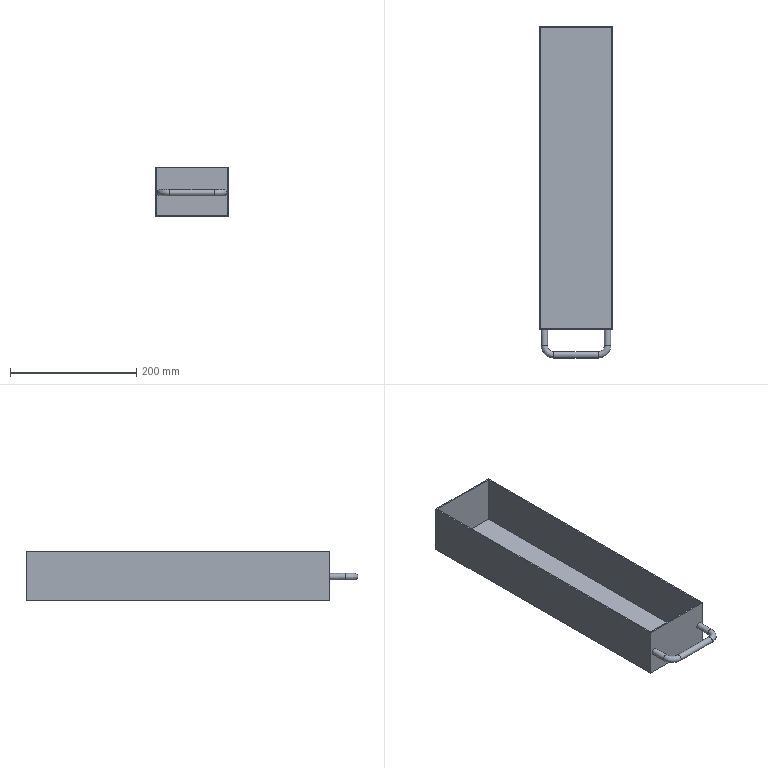Part | NX | features solid 2 | 1 solid | 16 faces | box 117 x 525 x 78 mm | volume 305718 mm3 | plane 11 | cylinder 3 | torus 2 | commonest cylinder face diameters 10 x3
STEP:
#1=CARTESIAN_POINT('',(-337.5,-405.,-285.));
#2=VERTEX_POINT('',#1);
#3=CARTESIAN_POINT('',(-337.5,-405.,-280.));
#4=DIRECTION('',(0.,-1.,0.));
#5=DIRECTION('',(0.,0.,-1.));
#6=AXIS2_PLACEMENT_3D('',#3,#4,#5);
#7=CIRCLE('',#6,5.);
#8=EDGE_CURVE('',#2,#2,#7,.T.);
#9=ORIENTED_EDGE('',*,*,#8,.F.);
#10=EDGE_LOOP('',(#9));
#11=FACE_BOUND('',#10,.T.);
#12=CARTESIAN_POINT('',(-346.,-405.,-240.));
#13=VERTEX_POINT('',#12);
#14=CARTESIAN_POINT('',(-229.,-405.,-240.));
#15=VERTEX_POINT('',#14);
#16=CARTESIAN_POINT('',(-350.,-405.,-240.));
#17=DIRECTION('',(1.,0.,0.));
#18=VECTOR('',#17,1000.);
#19=LINE('',#16,#18);
#20=EDGE_CURVE('',#13,#15,#19,.T.);
#21=ORIENTED_EDGE('',*,*,#20,.F.);
#22=CARTESIAN_POINT('',(-346.,-405.,-318.));
#23=VERTEX_POINT('',#22);
#24=CARTESIAN_POINT('',(-346.,-405.,0.));
#25=DIRECTION('',(0.,0.,1.));
#26=VECTOR('',#25,1000.);
#27=LINE('',#24,#26);
#28=EDGE_CURVE('',#23,#13,#27,.T.);
#29=ORIENTED_EDGE('',*,*,#28,.F.);
#30=CARTESIAN_POINT('',(-229.,-405.,-318.));
#31=VERTEX_POINT('',#30);
#32=CARTESIAN_POINT('',(-350.,-405.,-318.));
#33=DIRECTION('',(-1.,0.,0.));
#34=VECTOR('',#33,1000.);
#35=LINE('',#32,#34);
#36=EDGE_CURVE('',#23,#31,#35,.F.);
#37=ORIENTED_EDGE('',*,*,#36,.T.);
#38=CARTESIAN_POINT('',(-229.,-405.,-85.));
#39=DIRECTION('',(0.,0.,1.));
#40=VECTOR('',#39,1000.);
#41=LINE('',#38,#40);
#42=EDGE_CURVE('',#31,#15,#41,.T.);
#43=ORIENTED_EDGE('',*,*,#42,.T.);
#44=EDGE_LOOP('',(#21,#29,#37,#43));
#45=FACE_BOUND('',#44,.T.);
#46=CARTESIAN_POINT('',(-242.5,-405.,-280.));
#47=VERTEX_POINT('',#46);
#48=CARTESIAN_POINT('',(-237.5,-405.,-280.));
#49=DIRECTION('',(0.,-1.,0.));
#50=DIRECTION('',(-1.,0.,0.));
#51=AXIS2_PLACEMENT_3D('',#48,#49,#50);
#52=CIRCLE('',#51,5.);
#53=EDGE_CURVE('',#47,#47,#52,.T.);
#54=ORIENTED_EDGE('',*,*,#53,.F.);
#55=EDGE_LOOP('',(#54));
#56=FACE_BOUND('',#55,.T.);
#57=CARTESIAN_POINT('',(-910.,-405.,-85.));
#58=DIRECTION('',(0.,-1.,0.));
#59=DIRECTION('',(0.,0.,-1.));
#60=AXIS2_PLACEMENT_3D('',#57,#58,#59);
#61=PLANE('',#60);
#62=ADVANCED_FACE('',(#11,#45,#56),#61,.T.);
#63=CARTESIAN_POINT('',(-229.,75.,-240.));
#64=VERTEX_POINT('',#63);
#65=CARTESIAN_POINT('',(-346.,75.,-240.));
#66=VERTEX_POINT('',#65);
#67=CARTESIAN_POINT('',(-350.,75.,-240.));
#68=DIRECTION('',(1.,0.,0.));
#69=VECTOR('',#68,1000.);
#70=LINE('',#67,#69);
#71=EDGE_CURVE('',#64,#66,#70,.F.);
#72=ORIENTED_EDGE('',*,*,#71,.F.);
#73=CARTESIAN_POINT('',(-229.,75.,-318.));
#74=VERTEX_POINT('',#73);
#75=CARTESIAN_POINT('',(-229.,75.,0.));
#76=DIRECTION('',(0.,0.,-1.));
#77=VECTOR('',#76,1000.);
#78=LINE('',#75,#77);
#79=EDGE_CURVE('',#74,#64,#78,.F.);
#80=ORIENTED_EDGE('',*,*,#79,.F.);
#81=CARTESIAN_POINT('',(-346.,75.,-318.));
#82=VERTEX_POINT('',#81);
#83=CARTESIAN_POINT('',(-350.,75.,-318.));
#84=DIRECTION('',(-1.,0.,0.));
#85=VECTOR('',#84,1000.);
#86=LINE('',#83,#85);
#87=EDGE_CURVE('',#74,#82,#86,.T.);
#88=ORIENTED_EDGE('',*,*,#87,.T.);
#89=CARTESIAN_POINT('',(-346.,75.,-320.));
#90=DIRECTION('',(0.,0.,-1.));
#91=VECTOR('',#90,1000.);
#92=LINE('',#89,#91);
#93=EDGE_CURVE('',#82,#66,#92,.F.);
#94=ORIENTED_EDGE('',*,*,#93,.T.);
#95=EDGE_LOOP('',(#72,#80,#88,#94));
#96=FACE_BOUND('',#95,.T.);
#97=CARTESIAN_POINT('',(-225.,75.,-320.));
#98=DIRECTION('',(0.,-1.,0.));
#99=DIRECTION('',(-1.,0.,0.));
#100=AXIS2_PLACEMENT_3D('',#97,#98,#99);
#101=PLANE('',#100);
#102=ADVANCED_FACE('',(#96),#101,.F.);
#103=CARTESIAN_POINT('',(-346.,105.,-240.));
#104=DIRECTION('',(0.,-1.,0.));
#105=VECTOR('',#104,1000.);
#106=LINE('',#103,#105);
#107=EDGE_CURVE('',#66,#13,#106,.T.);
#108=ORIENTED_EDGE('',*,*,#107,.F.);
#109=ORIENTED_EDGE('',*,*,#93,.F.);
#110=CARTESIAN_POINT('',(-346.,-70.,-318.));
#111=DIRECTION('',(0.,1.,0.));
#112=VECTOR('',#111,1000.);
#113=LINE('',#110,#112);
#114=EDGE_CURVE('',#82,#23,#113,.F.);
#115=ORIENTED_EDGE('',*,*,#114,.T.);
#116=ORIENTED_EDGE('',*,*,#28,.T.);
#117=EDGE_LOOP('',(#108,#109,#115,#116));
#118=FACE_BOUND('',#117,.T.);
#119=CARTESIAN_POINT('',(-346.,105.,0.));
#120=DIRECTION('',(-1.,0.,0.));
#121=DIRECTION('',(0.,0.,1.));
#122=AXIS2_PLACEMENT_3D('',#119,#120,#121);
#123=PLANE('',#122);
#124=ADVANCED_FACE('',(#118),#123,.T.);
#125=CARTESIAN_POINT('',(-229.,105.,-240.));
#126=DIRECTION('',(0.,1.,0.));
#127=VECTOR('',#126,1000.);
#128=LINE('',#125,#127);
#129=EDGE_CURVE('',#15,#64,#128,.T.);
#130=ORIENTED_EDGE('',*,*,#129,.F.);
#131=ORIENTED_EDGE('',*,*,#42,.F.);
#132=CARTESIAN_POINT('',(-229.,-70.,-318.));
#133=DIRECTION('',(0.,-1.,0.));
#134=VECTOR('',#133,1000.);
#135=LINE('',#132,#134);
#136=EDGE_CURVE('',#31,#74,#135,.F.);
#137=ORIENTED_EDGE('',*,*,#136,.T.);
#138=ORIENTED_EDGE('',*,*,#79,.T.);
#139=EDGE_LOOP('',(#130,#131,#137,#138));
#140=FACE_BOUND('',#139,.T.);
#141=CARTESIAN_POINT('',(-229.,-400.,0.));
#142=DIRECTION('',(1.,0.,0.));
#143=DIRECTION('',(0.,0.,-1.));
#144=AXIS2_PLACEMENT_3D('',#141,#142,#143);
#145=PLANE('',#144);
#146=ADVANCED_FACE('',(#140),#145,.T.);
#147=ORIENTED_EDGE('',*,*,#87,.F.);
#148=ORIENTED_EDGE('',*,*,#136,.F.);
#149=ORIENTED_EDGE('',*,*,#36,.F.);
#150=ORIENTED_EDGE('',*,*,#114,.F.);
#151=EDGE_LOOP('',(#147,#148,#149,#150));
#152=FACE_BOUND('',#151,.T.);
#153=CARTESIAN_POINT('',(-350.,-70.,-318.));
#154=DIRECTION('',(0.,0.,-1.));
#155=DIRECTION('',(-1.,0.,0.));
#156=AXIS2_PLACEMENT_3D('',#153,#154,#155);
#157=PLANE('',#156);
#158=ADVANCED_FACE('',(#152),#157,.T.);
#159=CARTESIAN_POINT('',(-231.,73.,-240.));
#160=VERTEX_POINT('',#159);
#161=CARTESIAN_POINT('',(-344.,73.,-240.));
#162=VERTEX_POINT('',#161);
#163=CARTESIAN_POINT('',(-350.,73.,-240.));
#164=DIRECTION('',(1.,0.,0.));
#165=VECTOR('',#164,1000.);
#166=LINE('',#163,#165);
#167=EDGE_CURVE('',#160,#162,#166,.F.);
#168=ORIENTED_EDGE('',*,*,#167,.F.);
#169=CARTESIAN_POINT('',(-231.,-403.,-240.));
#170=VERTEX_POINT('',#169);
#171=CARTESIAN_POINT('',(-231.,105.,-240.));
#172=DIRECTION('',(0.,1.,0.));
#173=VECTOR('',#172,1000.);
#174=LINE('',#171,#173);
#175=EDGE_CURVE('',#170,#160,#174,.T.);
#176=ORIENTED_EDGE('',*,*,#175,.F.);
#177=CARTESIAN_POINT('',(-344.,-403.,-240.));
#178=VERTEX_POINT('',#177);
#179=CARTESIAN_POINT('',(-350.,-403.,-240.));
#180=DIRECTION('',(1.,0.,0.));
#181=VECTOR('',#180,1000.);
#182=LINE('',#179,#181);
#183=EDGE_CURVE('',#178,#170,#182,.T.);
#184=ORIENTED_EDGE('',*,*,#183,.F.);
#185=CARTESIAN_POINT('',(-344.,105.,-240.));
#186=DIRECTION('',(0.,-1.,0.));
#187=VECTOR('',#186,1000.);
#188=LINE('',#185,#187);
#189=EDGE_CURVE('',#162,#178,#188,.T.);
#190=ORIENTED_EDGE('',*,*,#189,.F.);
#191=EDGE_LOOP('',(#168,#176,#184,#190));
#192=FACE_BOUND('',#191,.T.);
#193=ORIENTED_EDGE('',*,*,#71,.T.);
#194=ORIENTED_EDGE('',*,*,#107,.T.);
#195=ORIENTED_EDGE('',*,*,#20,.T.);
#196=ORIENTED_EDGE('',*,*,#129,.T.);
#197=EDGE_LOOP('',(#193,#194,#195,#196));
#198=FACE_BOUND('',#197,.T.);
#199=CARTESIAN_POINT('',(-350.,105.,-240.));
#200=DIRECTION('',(0.,0.,1.));
#201=DIRECTION('',(1.,0.,0.));
#202=AXIS2_PLACEMENT_3D('',#199,#200,#201);
#203=PLANE('',#202);
#204=ADVANCED_FACE('',(#192,#198),#203,.T.);
#205=ORIENTED_EDGE('',*,*,#167,.T.);
#206=CARTESIAN_POINT('',(-344.,73.,-316.));
#207=VERTEX_POINT('',#206);
#208=CARTESIAN_POINT('',(-344.,73.,-320.));
#209=DIRECTION('',(0.,0.,-1.));
#210=VECTOR('',#209,1000.);
#211=LINE('',#208,#210);
#212=EDGE_CURVE('',#207,#162,#211,.F.);
#213=ORIENTED_EDGE('',*,*,#212,.F.);
#214=CARTESIAN_POINT('',(-231.,73.,-316.));
#215=VERTEX_POINT('',#214);
#216=CARTESIAN_POINT('',(-350.,73.,-316.));
#217=DIRECTION('',(-1.,0.,0.));
#218=VECTOR('',#217,1000.);
#219=LINE('',#216,#218);
#220=EDGE_CURVE('',#215,#207,#219,.T.);
#221=ORIENTED_EDGE('',*,*,#220,.F.);
#222=CARTESIAN_POINT('',(-231.,73.,0.));
#223=DIRECTION('',(0.,0.,-1.));
#224=VECTOR('',#223,1000.);
#225=LINE('',#222,#224);
#226=EDGE_CURVE('',#215,#160,#225,.F.);
#227=ORIENTED_EDGE('',*,*,#226,.T.);
#228=EDGE_LOOP('',(#205,#213,#221,#227));
#229=FACE_BOUND('',#228,.T.);
#230=CARTESIAN_POINT('',(-225.,73.,-320.));
#231=DIRECTION('',(0.,-1.,0.));
#232=DIRECTION('',(-1.,0.,0.));
#233=AXIS2_PLACEMENT_3D('',#230,#231,#232);
#234=PLANE('',#233);
#235=ADVANCED_FACE('',(#229),#234,.T.);
#236=ORIENTED_EDGE('',*,*,#189,.T.);
#237=CARTESIAN_POINT('',(-344.,-403.,-316.));
#238=VERTEX_POINT('',#237);
#239=CARTESIAN_POINT('',(-344.,-403.,0.));
#240=DIRECTION('',(0.,0.,1.));
#241=VECTOR('',#240,1000.);
#242=LINE('',#239,#241);
#243=EDGE_CURVE('',#238,#178,#242,.T.);
#244=ORIENTED_EDGE('',*,*,#243,.F.);
#245=CARTESIAN_POINT('',(-344.,-70.,-316.));
#246=DIRECTION('',(0.,1.,0.));
#247=VECTOR('',#246,1000.);
#248=LINE('',#245,#247);
#249=EDGE_CURVE('',#207,#238,#248,.F.);
#250=ORIENTED_EDGE('',*,*,#249,.F.);
#251=ORIENTED_EDGE('',*,*,#212,.T.);
#252=EDGE_LOOP('',(#236,#244,#250,#251));
#253=FACE_BOUND('',#252,.T.);
#254=CARTESIAN_POINT('',(-344.,105.,0.));
#255=DIRECTION('',(-1.,0.,0.));
#256=DIRECTION('',(0.,0.,1.));
#257=AXIS2_PLACEMENT_3D('',#254,#255,#256);
#258=PLANE('',#257);
#259=ADVANCED_FACE('',(#253),#258,.F.);
#260=ORIENTED_EDGE('',*,*,#183,.T.);
#261=CARTESIAN_POINT('',(-231.,-403.,-316.));
#262=VERTEX_POINT('',#261);
#263=CARTESIAN_POINT('',(-231.,-403.,-85.));
#264=DIRECTION('',(0.,0.,1.));
#265=VECTOR('',#264,1000.);
#266=LINE('',#263,#265);
#267=EDGE_CURVE('',#262,#170,#266,.T.);
#268=ORIENTED_EDGE('',*,*,#267,.F.);
#269=CARTESIAN_POINT('',(-350.,-403.,-316.));
#270=DIRECTION('',(-1.,0.,0.));
#271=VECTOR('',#270,1000.);
#272=LINE('',#269,#271);
#273=EDGE_CURVE('',#238,#262,#272,.F.);
#274=ORIENTED_EDGE('',*,*,#273,.F.);
#275=ORIENTED_EDGE('',*,*,#243,.T.);
#276=EDGE_LOOP('',(#260,#268,#274,#275));
#277=FACE_BOUND('',#276,.T.);
#278=CARTESIAN_POINT('',(-910.,-403.,-85.));
#279=DIRECTION('',(0.,-1.,0.));
#280=DIRECTION('',(0.,0.,-1.));
#281=AXIS2_PLACEMENT_3D('',#278,#279,#280);
#282=PLANE('',#281);
#283=ADVANCED_FACE('',(#277),#282,.F.);
#284=ORIENTED_EDGE('',*,*,#175,.T.);
#285=ORIENTED_EDGE('',*,*,#226,.F.);
#286=CARTESIAN_POINT('',(-231.,-70.,-316.));
#287=DIRECTION('',(0.,-1.,0.));
#288=VECTOR('',#287,1000.);
#289=LINE('',#286,#288);
#290=EDGE_CURVE('',#262,#215,#289,.F.);
#291=ORIENTED_EDGE('',*,*,#290,.F.);
#292=ORIENTED_EDGE('',*,*,#267,.T.);
#293=EDGE_LOOP('',(#284,#285,#291,#292));
#294=FACE_BOUND('',#293,.T.);
#295=CARTESIAN_POINT('',(-231.,-400.,0.));
#296=DIRECTION('',(1.,0.,0.));
#297=DIRECTION('',(0.,0.,-1.));
#298=AXIS2_PLACEMENT_3D('',#295,#296,#297);
#299=PLANE('',#298);
#300=ADVANCED_FACE('',(#294),#299,.F.);
#301=ORIENTED_EDGE('',*,*,#220,.T.);
#302=ORIENTED_EDGE('',*,*,#249,.T.);
#303=ORIENTED_EDGE('',*,*,#273,.T.);
#304=ORIENTED_EDGE('',*,*,#290,.T.);
#305=EDGE_LOOP('',(#301,#302,#303,#304));
#306=FACE_BOUND('',#305,.T.);
#307=CARTESIAN_POINT('',(-350.,-70.,-316.));
#308=DIRECTION('',(0.,0.,-1.));
#309=DIRECTION('',(-1.,0.,0.));
#310=AXIS2_PLACEMENT_3D('',#307,#308,#309);
#311=PLANE('',#310);
#312=ADVANCED_FACE('',(#306),#311,.F.);
#313=CARTESIAN_POINT('',(-242.5,-430.,-280.));
#314=VERTEX_POINT('',#313);
#315=CARTESIAN_POINT('',(-237.5,-430.,-280.));
#316=DIRECTION('',(0.,-1.,0.));
#317=DIRECTION('',(-1.,0.,0.));
#318=AXIS2_PLACEMENT_3D('',#315,#316,#317);
#319=CIRCLE('',#318,5.);
#320=EDGE_CURVE('',#314,#314,#319,.T.);
#321=ORIENTED_EDGE('',*,*,#320,.F.);
#322=EDGE_LOOP('',(#321));
#323=FACE_BOUND('',#322,.T.);
#324=ORIENTED_EDGE('',*,*,#53,.T.);
#325=EDGE_LOOP('',(#324));
#326=FACE_BOUND('',#325,.T.);
#327=CARTESIAN_POINT('',(-237.5,-430.,-280.));
#328=DIRECTION('',(0.,1.,0.));
#329=DIRECTION('',(0.,0.,1.));
#330=AXIS2_PLACEMENT_3D('',#327,#328,#329);
#331=CYLINDRICAL_SURFACE('',#330,5.);
#332=ADVANCED_FACE('',(#323,#326),#331,.T.);
#333=CARTESIAN_POINT('',(-252.5,-440.,-280.));
#334=VERTEX_POINT('',#333);
#335=CARTESIAN_POINT('',(-252.5,-445.,-280.));
#336=DIRECTION('',(-1.,0.,0.));
#337=DIRECTION('',(0.,1.,0.));
#338=AXIS2_PLACEMENT_3D('',#335,#336,#337);
#339=CIRCLE('',#338,5.);
#340=EDGE_CURVE('',#334,#334,#339,.T.);
#341=ORIENTED_EDGE('',*,*,#340,.F.);
#342=EDGE_LOOP('',(#341));
#343=FACE_BOUND('',#342,.T.);
#344=ORIENTED_EDGE('',*,*,#320,.T.);
#345=EDGE_LOOP('',(#344));
#346=FACE_BOUND('',#345,.T.);
#347=CARTESIAN_POINT('',(-252.5,-430.,-280.));
#348=DIRECTION('',(0.,0.,1.));
#349=DIRECTION('',(1.,0.,0.));
#350=AXIS2_PLACEMENT_3D('',#347,#348,#349);
#351=TOROIDAL_SURFACE('',#350,15.,5.);
#352=ADVANCED_FACE('',(#343,#346),#351,.T.);
#353=ORIENTED_EDGE('',*,*,#340,.T.);
#354=EDGE_LOOP('',(#353));
#355=FACE_BOUND('',#354,.T.);
#356=CARTESIAN_POINT('',(-322.5,-440.,-280.));
#357=VERTEX_POINT('',#356);
#358=CARTESIAN_POINT('',(-322.5,-445.,-280.));
#359=DIRECTION('',(-1.,0.,0.));
#360=DIRECTION('',(0.,1.,0.));
#361=AXIS2_PLACEMENT_3D('',#358,#359,#360);
#362=CIRCLE('',#361,5.);
#363=EDGE_CURVE('',#357,#357,#362,.T.);
#364=ORIENTED_EDGE('',*,*,#363,.F.);
#365=EDGE_LOOP('',(#364));
#366=FACE_BOUND('',#365,.T.);
#367=CARTESIAN_POINT('',(-322.5,-445.,-280.));
#368=DIRECTION('',(1.,0.,0.));
#369=DIRECTION('',(0.,0.,-1.));
#370=AXIS2_PLACEMENT_3D('',#367,#368,#369);
#371=CYLINDRICAL_SURFACE('',#370,5.);
#372=ADVANCED_FACE('',(#355,#366),#371,.T.);
#373=CARTESIAN_POINT('',(-332.5,-430.,-280.));
#374=VERTEX_POINT('',#373);
#375=CARTESIAN_POINT('',(-337.5,-430.,-280.));
#376=DIRECTION('',(0.,1.,0.));
#377=DIRECTION('',(1.,0.,0.));
#378=AXIS2_PLACEMENT_3D('',#375,#376,#377);
#379=CIRCLE('',#378,5.);
#380=EDGE_CURVE('',#374,#374,#379,.T.);
#381=ORIENTED_EDGE('',*,*,#380,.F.);
#382=EDGE_LOOP('',(#381));
#383=FACE_BOUND('',#382,.T.);
#384=ORIENTED_EDGE('',*,*,#363,.T.);
#385=EDGE_LOOP('',(#384));
#386=FACE_BOUND('',#385,.T.);
#387=CARTESIAN_POINT('',(-322.5,-430.,-280.));
#388=DIRECTION('',(0.,0.,1.));
#389=DIRECTION('',(1.,0.,0.));
#390=AXIS2_PLACEMENT_3D('',#387,#388,#389);
#391=TOROIDAL_SURFACE('',#390,15.,5.);
#392=ADVANCED_FACE('',(#383,#386),#391,.T.);
#393=ORIENTED_EDGE('',*,*,#380,.T.);
#394=EDGE_LOOP('',(#393));
#395=FACE_BOUND('',#394,.T.);
#396=ORIENTED_EDGE('',*,*,#8,.T.);
#397=EDGE_LOOP('',(#396));
#398=FACE_BOUND('',#397,.T.);
#399=CARTESIAN_POINT('',(-337.5,-430.,-280.));
#400=DIRECTION('',(0.,1.,0.));
#401=DIRECTION('',(0.,0.,1.));
#402=AXIS2_PLACEMENT_3D('',#399,#400,#401);
#403=CYLINDRICAL_SURFACE('',#402,5.);
#404=ADVANCED_FACE('',(#395,#398),#403,.T.);
#405=CLOSED_SHELL('',(#62,#102,#124,#146,#158,#204,#235,#259,#283,#300,#312,#332,#352,#372,#392,#404));
#406=MANIFOLD_SOLID_BREP('',#405);
#407=(LENGTH_UNIT()NAMED_UNIT(*)SI_UNIT(.MILLI.,.METRE.));
#408=UNCERTAINTY_MEASURE_WITH_UNIT(LENGTH_MEASURE(0.00001),#407,'','');
#409=(NAMED_UNIT(*)PLANE_ANGLE_UNIT()SI_UNIT($,.RADIAN.));
#410=(NAMED_UNIT(*)SI_UNIT($,.STERADIAN.)SOLID_ANGLE_UNIT());
#411=(GEOMETRIC_REPRESENTATION_CONTEXT(3)GLOBAL_UNCERTAINTY_ASSIGNED_CONTEXT((#408))GLOBAL_UNIT_ASSIGNED_CONTEXT((#407,#409,#410))REPRESENTATION_CONTEXT('',''));
#412=ADVANCED_BREP_SHAPE_REPRESENTATION('',(#406),#411);